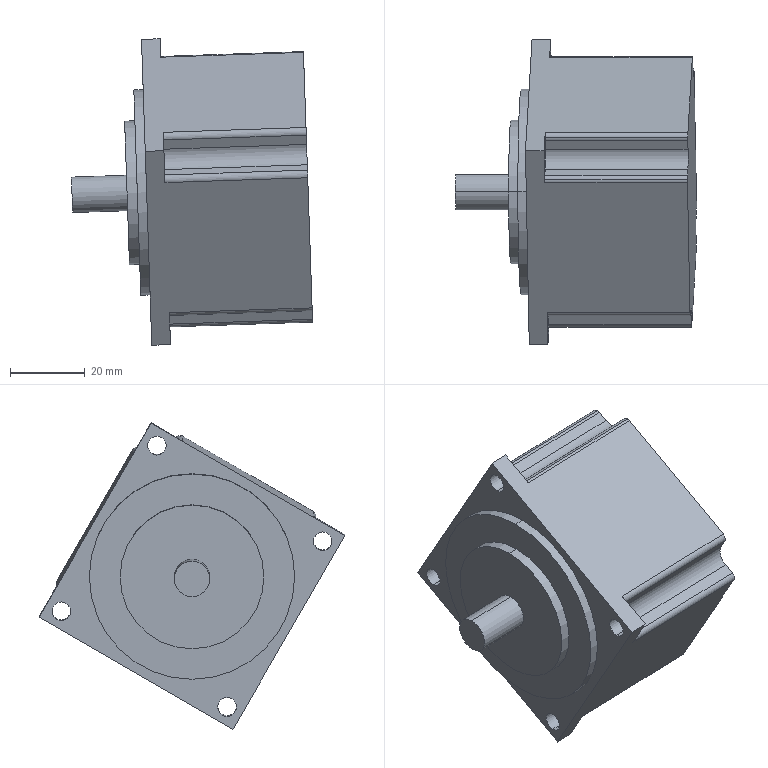Part | STEP file | 2026.6.15-Main Assembly图.sldasm-Part-85 | 1 solid | 50 faces | box 64.6 x 81.962 x 82.084 mm | volume 155159 mm3 | cylinder 29 | plane 21 | commonest cylinder face diameters 3 x10 5 x8 8 x5 9.5 x2 38.5 x2 55 x2